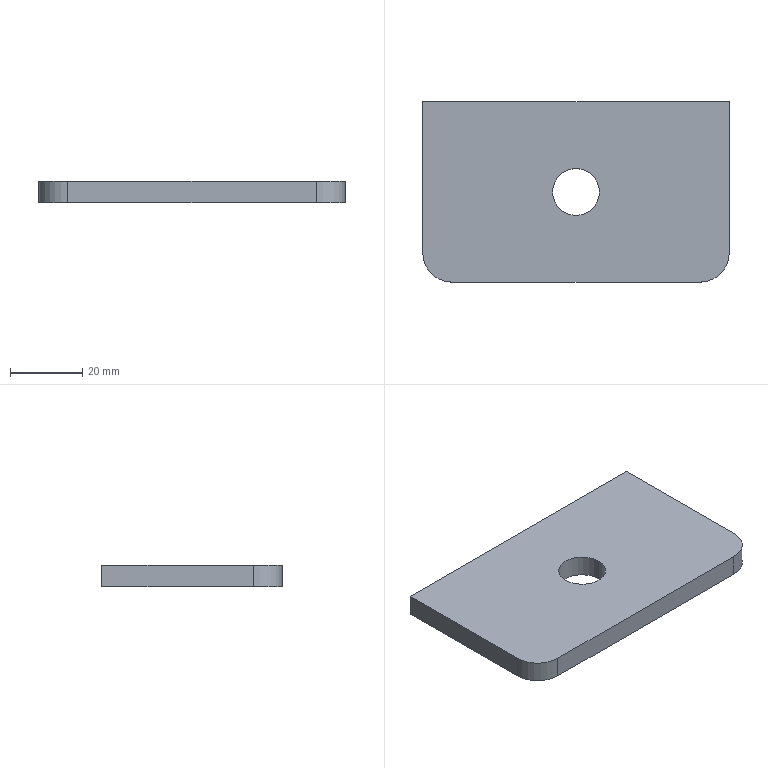Part | SolidWorks | features Extrusion 1 | 1 solid | 10 faces | box 85 x 50 x 6 mm | volume 24539 mm3 | plane 6 | cylinder 4 | commonest cylinder face diameters 13 x2 16 x2
STEP:
#1=CARTESIAN_POINT('',(-6.5,0.,6.));
#2=VERTEX_POINT('',#1);
#3=CARTESIAN_POINT('',(6.5,0.,6.));
#4=VERTEX_POINT('',#3);
#5=CARTESIAN_POINT('',(0.,0.,6.));
#6=DIRECTION('',(0.,0.,1.));
#7=DIRECTION('',(1.,0.,0.));
#8=AXIS2_PLACEMENT_3D('',#5,#6,#7);
#9=CIRCLE('',#8,6.5);
#10=EDGE_CURVE('',#2,#4,#9,.T.);
#11=ORIENTED_EDGE('',*,*,#10,.T.);
#12=CARTESIAN_POINT('',(6.5,0.,0.));
#13=VERTEX_POINT('',#12);
#14=CARTESIAN_POINT('',(6.5,0.,6.));
#15=DIRECTION('',(0.,0.,-1.));
#16=VECTOR('',#15,1000.);
#17=LINE('',#14,#16);
#18=EDGE_CURVE('',#4,#13,#17,.T.);
#19=ORIENTED_EDGE('',*,*,#18,.T.);
#20=CARTESIAN_POINT('',(-6.5,0.,0.));
#21=VERTEX_POINT('',#20);
#22=CARTESIAN_POINT('',(0.,0.,0.));
#23=DIRECTION('',(0.,0.,1.));
#24=DIRECTION('',(1.,0.,0.));
#25=AXIS2_PLACEMENT_3D('',#22,#23,#24);
#26=CIRCLE('',#25,6.5);
#27=EDGE_CURVE('',#21,#13,#26,.T.);
#28=ORIENTED_EDGE('',*,*,#27,.F.);
#29=CARTESIAN_POINT('',(-6.5,0.,6.));
#30=DIRECTION('',(0.,0.,-1.));
#31=VECTOR('',#30,1000.);
#32=LINE('',#29,#31);
#33=EDGE_CURVE('',#2,#21,#32,.T.);
#34=ORIENTED_EDGE('',*,*,#33,.F.);
#35=EDGE_LOOP('',(#11,#19,#28,#34));
#36=FACE_OUTER_BOUND('',#35,.T.);
#37=CARTESIAN_POINT('',(0.,0.,6.));
#38=DIRECTION('',(0.,0.,-1.));
#39=DIRECTION('',(-1.,0.,0.));
#40=AXIS2_PLACEMENT_3D('',#37,#38,#39);
#41=CYLINDRICAL_SURFACE('',#40,6.5);
#42=ADVANCED_FACE('',(#36),#41,.F.);
#43=CARTESIAN_POINT('',(-42.5,25.,6.));
#44=VERTEX_POINT('',#43);
#45=CARTESIAN_POINT('',(-42.5,-17.,6.));
#46=VERTEX_POINT('',#45);
#47=CARTESIAN_POINT('',(-42.5,25.,6.));
#48=DIRECTION('',(0.,-1.,0.));
#49=VECTOR('',#48,1000.);
#50=LINE('',#47,#49);
#51=EDGE_CURVE('',#44,#46,#50,.T.);
#52=ORIENTED_EDGE('',*,*,#51,.T.);
#53=CARTESIAN_POINT('',(-34.5,-25.,6.));
#54=VERTEX_POINT('',#53);
#55=CARTESIAN_POINT('',(-34.5,-17.,6.));
#56=DIRECTION('',(0.,0.,1.));
#57=DIRECTION('',(1.,0.,0.));
#58=AXIS2_PLACEMENT_3D('',#55,#56,#57);
#59=CIRCLE('',#58,8.);
#60=EDGE_CURVE('',#46,#54,#59,.T.);
#61=ORIENTED_EDGE('',*,*,#60,.T.);
#62=CARTESIAN_POINT('',(34.5,-25.,6.));
#63=VERTEX_POINT('',#62);
#64=CARTESIAN_POINT('',(-34.5,-25.,6.));
#65=DIRECTION('',(1.,0.,0.));
#66=VECTOR('',#65,1000.);
#67=LINE('',#64,#66);
#68=EDGE_CURVE('',#54,#63,#67,.T.);
#69=ORIENTED_EDGE('',*,*,#68,.T.);
#70=CARTESIAN_POINT('',(42.5,-17.,6.));
#71=VERTEX_POINT('',#70);
#72=CARTESIAN_POINT('',(34.5,-17.,6.));
#73=DIRECTION('',(0.,0.,1.));
#74=DIRECTION('',(1.,0.,0.));
#75=AXIS2_PLACEMENT_3D('',#72,#73,#74);
#76=CIRCLE('',#75,8.);
#77=EDGE_CURVE('',#63,#71,#76,.T.);
#78=ORIENTED_EDGE('',*,*,#77,.T.);
#79=CARTESIAN_POINT('',(42.5,25.,6.));
#80=VERTEX_POINT('',#79);
#81=CARTESIAN_POINT('',(42.5,25.,6.));
#82=DIRECTION('',(0.,1.,0.));
#83=VECTOR('',#82,1000.);
#84=LINE('',#81,#83);
#85=EDGE_CURVE('',#71,#80,#84,.T.);
#86=ORIENTED_EDGE('',*,*,#85,.T.);
#87=CARTESIAN_POINT('',(-42.5,25.,6.));
#88=DIRECTION('',(-1.,0.,0.));
#89=VECTOR('',#88,1000.);
#90=LINE('',#87,#89);
#91=EDGE_CURVE('',#80,#44,#90,.T.);
#92=ORIENTED_EDGE('',*,*,#91,.T.);
#93=EDGE_LOOP('',(#52,#61,#69,#78,#86,#92));
#94=FACE_OUTER_BOUND('',#93,.T.);
#95=ORIENTED_EDGE('',*,*,#10,.F.);
#96=CARTESIAN_POINT('',(0.,0.,6.));
#97=DIRECTION('',(0.,0.,1.));
#98=DIRECTION('',(1.,0.,0.));
#99=AXIS2_PLACEMENT_3D('',#96,#97,#98);
#100=CIRCLE('',#99,6.5);
#101=EDGE_CURVE('',#4,#2,#100,.T.);
#102=ORIENTED_EDGE('',*,*,#101,.F.);
#103=EDGE_LOOP('',(#95,#102));
#104=FACE_BOUND('',#103,.T.);
#105=CARTESIAN_POINT('',(-34.5,-17.,6.));
#106=DIRECTION('',(0.,0.,1.));
#107=DIRECTION('',(1.,0.,0.));
#108=AXIS2_PLACEMENT_3D('',#105,#106,#107);
#109=PLANE('',#108);
#110=ADVANCED_FACE('',(#94,#104),#109,.T.);
#111=CARTESIAN_POINT('',(-42.5,25.,0.));
#112=VERTEX_POINT('',#111);
#113=CARTESIAN_POINT('',(-42.5,-17.,0.));
#114=VERTEX_POINT('',#113);
#115=CARTESIAN_POINT('',(-42.5,25.,0.));
#116=DIRECTION('',(0.,-1.,0.));
#117=VECTOR('',#116,1000.);
#118=LINE('',#115,#117);
#119=EDGE_CURVE('',#112,#114,#118,.T.);
#120=ORIENTED_EDGE('',*,*,#119,.F.);
#121=CARTESIAN_POINT('',(42.5,25.,0.));
#122=VERTEX_POINT('',#121);
#123=CARTESIAN_POINT('',(-42.5,25.,0.));
#124=DIRECTION('',(-1.,0.,0.));
#125=VECTOR('',#124,1000.);
#126=LINE('',#123,#125);
#127=EDGE_CURVE('',#122,#112,#126,.T.);
#128=ORIENTED_EDGE('',*,*,#127,.F.);
#129=CARTESIAN_POINT('',(42.5,-17.,0.));
#130=VERTEX_POINT('',#129);
#131=CARTESIAN_POINT('',(42.5,25.,0.));
#132=DIRECTION('',(0.,1.,0.));
#133=VECTOR('',#132,1000.);
#134=LINE('',#131,#133);
#135=EDGE_CURVE('',#130,#122,#134,.T.);
#136=ORIENTED_EDGE('',*,*,#135,.F.);
#137=CARTESIAN_POINT('',(34.5,-25.,0.));
#138=VERTEX_POINT('',#137);
#139=CARTESIAN_POINT('',(34.5,-17.,0.));
#140=DIRECTION('',(0.,0.,1.));
#141=DIRECTION('',(1.,0.,0.));
#142=AXIS2_PLACEMENT_3D('',#139,#140,#141);
#143=CIRCLE('',#142,8.);
#144=EDGE_CURVE('',#138,#130,#143,.T.);
#145=ORIENTED_EDGE('',*,*,#144,.F.);
#146=CARTESIAN_POINT('',(-34.5,-25.,0.));
#147=VERTEX_POINT('',#146);
#148=CARTESIAN_POINT('',(-34.5,-25.,0.));
#149=DIRECTION('',(1.,0.,0.));
#150=VECTOR('',#149,1000.);
#151=LINE('',#148,#150);
#152=EDGE_CURVE('',#147,#138,#151,.T.);
#153=ORIENTED_EDGE('',*,*,#152,.F.);
#154=CARTESIAN_POINT('',(-34.5,-17.,0.));
#155=DIRECTION('',(0.,0.,1.));
#156=DIRECTION('',(1.,0.,0.));
#157=AXIS2_PLACEMENT_3D('',#154,#155,#156);
#158=CIRCLE('',#157,8.);
#159=EDGE_CURVE('',#114,#147,#158,.T.);
#160=ORIENTED_EDGE('',*,*,#159,.F.);
#161=EDGE_LOOP('',(#120,#128,#136,#145,#153,#160));
#162=FACE_OUTER_BOUND('',#161,.T.);
#163=ORIENTED_EDGE('',*,*,#27,.T.);
#164=CARTESIAN_POINT('',(0.,0.,0.));
#165=DIRECTION('',(0.,0.,1.));
#166=DIRECTION('',(1.,0.,0.));
#167=AXIS2_PLACEMENT_3D('',#164,#165,#166);
#168=CIRCLE('',#167,6.5);
#169=EDGE_CURVE('',#13,#21,#168,.T.);
#170=ORIENTED_EDGE('',*,*,#169,.T.);
#171=EDGE_LOOP('',(#163,#170));
#172=FACE_BOUND('',#171,.T.);
#173=CARTESIAN_POINT('',(-34.5,-17.,0.));
#174=DIRECTION('',(0.,0.,1.));
#175=DIRECTION('',(1.,0.,0.));
#176=AXIS2_PLACEMENT_3D('',#173,#174,#175);
#177=PLANE('',#176);
#178=ADVANCED_FACE('',(#162,#172),#177,.F.);
#179=ORIENTED_EDGE('',*,*,#119,.T.);
#180=CARTESIAN_POINT('',(-42.5,-17.,6.));
#181=DIRECTION('',(0.,0.,-1.));
#182=VECTOR('',#181,1000.);
#183=LINE('',#180,#182);
#184=EDGE_CURVE('',#46,#114,#183,.T.);
#185=ORIENTED_EDGE('',*,*,#184,.F.);
#186=ORIENTED_EDGE('',*,*,#51,.F.);
#187=CARTESIAN_POINT('',(-42.5,25.,6.));
#188=DIRECTION('',(0.,0.,-1.));
#189=VECTOR('',#188,1000.);
#190=LINE('',#187,#189);
#191=EDGE_CURVE('',#44,#112,#190,.T.);
#192=ORIENTED_EDGE('',*,*,#191,.T.);
#193=EDGE_LOOP('',(#179,#185,#186,#192));
#194=FACE_OUTER_BOUND('',#193,.T.);
#195=CARTESIAN_POINT('',(-42.5,25.,6.));
#196=DIRECTION('',(1.,0.,0.));
#197=DIRECTION('',(0.,1.,0.));
#198=AXIS2_PLACEMENT_3D('',#195,#196,#197);
#199=PLANE('',#198);
#200=ADVANCED_FACE('',(#194),#199,.F.);
#201=ORIENTED_EDGE('',*,*,#159,.T.);
#202=CARTESIAN_POINT('',(-34.5,-25.,6.));
#203=DIRECTION('',(0.,0.,-1.));
#204=VECTOR('',#203,1000.);
#205=LINE('',#202,#204);
#206=EDGE_CURVE('',#54,#147,#205,.T.);
#207=ORIENTED_EDGE('',*,*,#206,.F.);
#208=ORIENTED_EDGE('',*,*,#60,.F.);
#209=ORIENTED_EDGE('',*,*,#184,.T.);
#210=EDGE_LOOP('',(#201,#207,#208,#209));
#211=FACE_OUTER_BOUND('',#210,.T.);
#212=CARTESIAN_POINT('',(-34.5,-17.,6.));
#213=DIRECTION('',(0.,0.,-1.));
#214=DIRECTION('',(-1.,0.,0.));
#215=AXIS2_PLACEMENT_3D('',#212,#213,#214);
#216=CYLINDRICAL_SURFACE('',#215,8.);
#217=ADVANCED_FACE('',(#211),#216,.T.);
#218=ORIENTED_EDGE('',*,*,#152,.T.);
#219=CARTESIAN_POINT('',(34.5,-25.,6.));
#220=DIRECTION('',(0.,0.,-1.));
#221=VECTOR('',#220,1000.);
#222=LINE('',#219,#221);
#223=EDGE_CURVE('',#63,#138,#222,.T.);
#224=ORIENTED_EDGE('',*,*,#223,.F.);
#225=ORIENTED_EDGE('',*,*,#68,.F.);
#226=ORIENTED_EDGE('',*,*,#206,.T.);
#227=EDGE_LOOP('',(#218,#224,#225,#226));
#228=FACE_OUTER_BOUND('',#227,.T.);
#229=CARTESIAN_POINT('',(-34.5,-25.,6.));
#230=DIRECTION('',(0.,1.,0.));
#231=DIRECTION('',(-1.,0.,0.));
#232=AXIS2_PLACEMENT_3D('',#229,#230,#231);
#233=PLANE('',#232);
#234=ADVANCED_FACE('',(#228),#233,.F.);
#235=ORIENTED_EDGE('',*,*,#144,.T.);
#236=CARTESIAN_POINT('',(42.5,-17.,6.));
#237=DIRECTION('',(0.,0.,-1.));
#238=VECTOR('',#237,1000.);
#239=LINE('',#236,#238);
#240=EDGE_CURVE('',#71,#130,#239,.T.);
#241=ORIENTED_EDGE('',*,*,#240,.F.);
#242=ORIENTED_EDGE('',*,*,#77,.F.);
#243=ORIENTED_EDGE('',*,*,#223,.T.);
#244=EDGE_LOOP('',(#235,#241,#242,#243));
#245=FACE_OUTER_BOUND('',#244,.T.);
#246=CARTESIAN_POINT('',(34.5,-17.,6.));
#247=DIRECTION('',(0.,0.,-1.));
#248=DIRECTION('',(-1.,0.,0.));
#249=AXIS2_PLACEMENT_3D('',#246,#247,#248);
#250=CYLINDRICAL_SURFACE('',#249,8.);
#251=ADVANCED_FACE('',(#245),#250,.T.);
#252=ORIENTED_EDGE('',*,*,#135,.T.);
#253=CARTESIAN_POINT('',(42.5,25.,6.));
#254=DIRECTION('',(0.,0.,-1.));
#255=VECTOR('',#254,1000.);
#256=LINE('',#253,#255);
#257=EDGE_CURVE('',#80,#122,#256,.T.);
#258=ORIENTED_EDGE('',*,*,#257,.F.);
#259=ORIENTED_EDGE('',*,*,#85,.F.);
#260=ORIENTED_EDGE('',*,*,#240,.T.);
#261=EDGE_LOOP('',(#252,#258,#259,#260));
#262=FACE_OUTER_BOUND('',#261,.T.);
#263=CARTESIAN_POINT('',(42.5,25.,6.));
#264=DIRECTION('',(-1.,0.,0.));
#265=DIRECTION('',(0.,-1.,0.));
#266=AXIS2_PLACEMENT_3D('',#263,#264,#265);
#267=PLANE('',#266);
#268=ADVANCED_FACE('',(#262),#267,.F.);
#269=ORIENTED_EDGE('',*,*,#127,.T.);
#270=ORIENTED_EDGE('',*,*,#191,.F.);
#271=ORIENTED_EDGE('',*,*,#91,.F.);
#272=ORIENTED_EDGE('',*,*,#257,.T.);
#273=EDGE_LOOP('',(#269,#270,#271,#272));
#274=FACE_OUTER_BOUND('',#273,.T.);
#275=CARTESIAN_POINT('',(-42.5,25.,6.));
#276=DIRECTION('',(0.,-1.,0.));
#277=DIRECTION('',(0.,0.,-1.));
#278=AXIS2_PLACEMENT_3D('',#275,#276,#277);
#279=PLANE('',#278);
#280=ADVANCED_FACE('',(#274),#279,.F.);
#281=ORIENTED_EDGE('',*,*,#18,.F.);
#282=ORIENTED_EDGE('',*,*,#101,.T.);
#283=ORIENTED_EDGE('',*,*,#33,.T.);
#284=ORIENTED_EDGE('',*,*,#169,.F.);
#285=EDGE_LOOP('',(#281,#282,#283,#284));
#286=FACE_OUTER_BOUND('',#285,.T.);
#287=CARTESIAN_POINT('',(0.,0.,6.));
#288=DIRECTION('',(0.,0.,-1.));
#289=DIRECTION('',(-1.,0.,0.));
#290=AXIS2_PLACEMENT_3D('',#287,#288,#289);
#291=CYLINDRICAL_SURFACE('',#290,6.5);
#292=ADVANCED_FACE('',(#286),#291,.F.);
#293=CLOSED_SHELL('',(#42,#110,#178,#200,#217,#234,#251,#268,#280,#292));
#294=MANIFOLD_SOLID_BREP('',#293);
#295=CARTESIAN_POINT('',(0.,0.,0.));
#296=DIRECTION('',(0.,0.,1.));
#297=DIRECTION('',(1.,0.,0.));
#298=AXIS2_PLACEMENT_3D('',#295,#296,#297);
#299=(LENGTH_UNIT()NAMED_UNIT(*)SI_UNIT(.MILLI.,.METRE.));
#300=UNCERTAINTY_MEASURE_WITH_UNIT(LENGTH_MEASURE(0.00001),#299,'','');
#301=(NAMED_UNIT(*)PLANE_ANGLE_UNIT()SI_UNIT($,.RADIAN.));
#302=(NAMED_UNIT(*)SI_UNIT($,.STERADIAN.)SOLID_ANGLE_UNIT());
#303=(GEOMETRIC_REPRESENTATION_CONTEXT(3)GLOBAL_UNCERTAINTY_ASSIGNED_CONTEXT((#300))GLOBAL_UNIT_ASSIGNED_CONTEXT((#299,#301,#302))REPRESENTATION_CONTEXT('',''));
#304=ADVANCED_BREP_SHAPE_REPRESENTATION('',(#294,#298),#303);